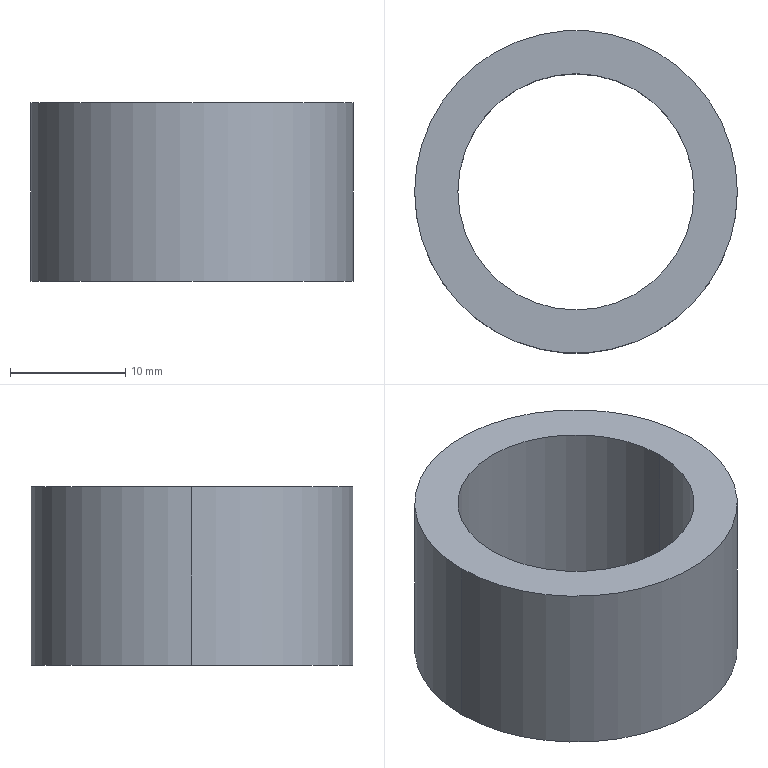Part | SolidWorks | features BaseBody 1 | 1 solid | 6 faces | box 28 x 28 x 15.5 mm | volume 4428 mm3 | cylinder 4 | plane 2 | commonest cylinder face diameters 20.5 x2 28 x2
STEP:
#1=CARTESIAN_POINT('',(10.25,0.,15.5));
#2=VERTEX_POINT('',#1);
#3=CARTESIAN_POINT('',(10.25,0.,0.));
#4=VERTEX_POINT('',#3);
#5=CARTESIAN_POINT('',(10.25,0.,15.5));
#6=DIRECTION('',(0.,0.,-1.));
#7=VECTOR('',#6,1000.);
#8=LINE('',#5,#7);
#9=EDGE_CURVE('',#2,#4,#8,.T.);
#10=ORIENTED_EDGE('',*,*,#9,.F.);
#11=CARTESIAN_POINT('',(-10.25,0.,15.5));
#12=VERTEX_POINT('',#11);
#13=CARTESIAN_POINT('',(0.,0.,15.5));
#14=DIRECTION('',(0.,0.,1.));
#15=DIRECTION('',(1.,0.,0.));
#16=AXIS2_PLACEMENT_3D('',#13,#14,#15);
#17=CIRCLE('',#16,10.25);
#18=EDGE_CURVE('',#2,#12,#17,.T.);
#19=ORIENTED_EDGE('',*,*,#18,.T.);
#20=CARTESIAN_POINT('',(-10.25,0.,0.));
#21=VERTEX_POINT('',#20);
#22=CARTESIAN_POINT('',(-10.25,0.,15.5));
#23=DIRECTION('',(0.,0.,-1.));
#24=VECTOR('',#23,1000.);
#25=LINE('',#22,#24);
#26=EDGE_CURVE('',#12,#21,#25,.T.);
#27=ORIENTED_EDGE('',*,*,#26,.T.);
#28=CARTESIAN_POINT('',(0.,0.,0.));
#29=DIRECTION('',(0.,0.,1.));
#30=DIRECTION('',(1.,0.,0.));
#31=AXIS2_PLACEMENT_3D('',#28,#29,#30);
#32=CIRCLE('',#31,10.25);
#33=EDGE_CURVE('',#4,#21,#32,.T.);
#34=ORIENTED_EDGE('',*,*,#33,.F.);
#35=EDGE_LOOP('',(#10,#19,#27,#34));
#36=FACE_OUTER_BOUND('',#35,.T.);
#37=CARTESIAN_POINT('',(0.,0.,15.5));
#38=DIRECTION('',(0.,0.,-1.));
#39=DIRECTION('',(-1.,0.,0.));
#40=AXIS2_PLACEMENT_3D('',#37,#38,#39);
#41=CYLINDRICAL_SURFACE('',#40,10.25);
#42=ADVANCED_FACE('',(#36),#41,.F.);
#43=CARTESIAN_POINT('',(14.,0.,15.5));
#44=VERTEX_POINT('',#43);
#45=CARTESIAN_POINT('',(14.,0.,0.));
#46=VERTEX_POINT('',#45);
#47=CARTESIAN_POINT('',(14.,0.,15.5));
#48=DIRECTION('',(0.,0.,-1.));
#49=VECTOR('',#48,1000.);
#50=LINE('',#47,#49);
#51=EDGE_CURVE('',#44,#46,#50,.T.);
#52=ORIENTED_EDGE('',*,*,#51,.F.);
#53=CARTESIAN_POINT('',(-14.,0.,15.5));
#54=VERTEX_POINT('',#53);
#55=CARTESIAN_POINT('',(0.,0.,15.5));
#56=DIRECTION('',(0.,0.,1.));
#57=DIRECTION('',(1.,0.,0.));
#58=AXIS2_PLACEMENT_3D('',#55,#56,#57);
#59=CIRCLE('',#58,14.);
#60=EDGE_CURVE('',#54,#44,#59,.T.);
#61=ORIENTED_EDGE('',*,*,#60,.F.);
#62=CARTESIAN_POINT('',(-14.,0.,0.));
#63=VERTEX_POINT('',#62);
#64=CARTESIAN_POINT('',(-14.,0.,15.5));
#65=DIRECTION('',(0.,0.,-1.));
#66=VECTOR('',#65,1000.);
#67=LINE('',#64,#66);
#68=EDGE_CURVE('',#54,#63,#67,.T.);
#69=ORIENTED_EDGE('',*,*,#68,.T.);
#70=CARTESIAN_POINT('',(0.,0.,0.));
#71=DIRECTION('',(0.,0.,1.));
#72=DIRECTION('',(1.,0.,0.));
#73=AXIS2_PLACEMENT_3D('',#70,#71,#72);
#74=CIRCLE('',#73,14.);
#75=EDGE_CURVE('',#63,#46,#74,.T.);
#76=ORIENTED_EDGE('',*,*,#75,.T.);
#77=EDGE_LOOP('',(#52,#61,#69,#76));
#78=FACE_OUTER_BOUND('',#77,.T.);
#79=CARTESIAN_POINT('',(0.,0.,15.5));
#80=DIRECTION('',(0.,0.,-1.));
#81=DIRECTION('',(-1.,0.,0.));
#82=AXIS2_PLACEMENT_3D('',#79,#80,#81);
#83=CYLINDRICAL_SURFACE('',#82,14.);
#84=ADVANCED_FACE('',(#78),#83,.T.);
#85=CARTESIAN_POINT('',(0.,0.,0.));
#86=DIRECTION('',(0.,0.,1.));
#87=DIRECTION('',(1.,0.,0.));
#88=AXIS2_PLACEMENT_3D('',#85,#86,#87);
#89=CIRCLE('',#88,10.25);
#90=EDGE_CURVE('',#21,#4,#89,.T.);
#91=ORIENTED_EDGE('',*,*,#90,.T.);
#92=ORIENTED_EDGE('',*,*,#33,.T.);
#93=EDGE_LOOP('',(#91,#92));
#94=FACE_BOUND('',#93,.T.);
#95=ORIENTED_EDGE('',*,*,#75,.F.);
#96=CARTESIAN_POINT('',(0.,0.,0.));
#97=DIRECTION('',(0.,0.,1.));
#98=DIRECTION('',(1.,0.,0.));
#99=AXIS2_PLACEMENT_3D('',#96,#97,#98);
#100=CIRCLE('',#99,14.);
#101=EDGE_CURVE('',#46,#63,#100,.T.);
#102=ORIENTED_EDGE('',*,*,#101,.F.);
#103=EDGE_LOOP('',(#95,#102));
#104=FACE_OUTER_BOUND('',#103,.T.);
#105=CARTESIAN_POINT('',(0.,0.,0.));
#106=DIRECTION('',(0.,0.,1.));
#107=DIRECTION('',(1.,0.,0.));
#108=AXIS2_PLACEMENT_3D('',#105,#106,#107);
#109=PLANE('',#108);
#110=ADVANCED_FACE('',(#94,#104),#109,.F.);
#111=CARTESIAN_POINT('',(0.,0.,15.5));
#112=DIRECTION('',(0.,0.,1.));
#113=DIRECTION('',(1.,0.,0.));
#114=AXIS2_PLACEMENT_3D('',#111,#112,#113);
#115=CIRCLE('',#114,10.25);
#116=EDGE_CURVE('',#12,#2,#115,.T.);
#117=ORIENTED_EDGE('',*,*,#116,.F.);
#118=ORIENTED_EDGE('',*,*,#18,.F.);
#119=EDGE_LOOP('',(#117,#118));
#120=FACE_BOUND('',#119,.T.);
#121=ORIENTED_EDGE('',*,*,#60,.T.);
#122=CARTESIAN_POINT('',(0.,0.,15.5));
#123=DIRECTION('',(0.,0.,1.));
#124=DIRECTION('',(1.,0.,0.));
#125=AXIS2_PLACEMENT_3D('',#122,#123,#124);
#126=CIRCLE('',#125,14.);
#127=EDGE_CURVE('',#44,#54,#126,.T.);
#128=ORIENTED_EDGE('',*,*,#127,.T.);
#129=EDGE_LOOP('',(#121,#128));
#130=FACE_OUTER_BOUND('',#129,.T.);
#131=CARTESIAN_POINT('',(0.,0.,15.5));
#132=DIRECTION('',(0.,0.,1.));
#133=DIRECTION('',(1.,0.,0.));
#134=AXIS2_PLACEMENT_3D('',#131,#132,#133);
#135=PLANE('',#134);
#136=ADVANCED_FACE('',(#120,#130),#135,.T.);
#137=ORIENTED_EDGE('',*,*,#127,.F.);
#138=ORIENTED_EDGE('',*,*,#51,.T.);
#139=ORIENTED_EDGE('',*,*,#101,.T.);
#140=ORIENTED_EDGE('',*,*,#68,.F.);
#141=EDGE_LOOP('',(#137,#138,#139,#140));
#142=FACE_OUTER_BOUND('',#141,.T.);
#143=CARTESIAN_POINT('',(0.,0.,15.5));
#144=DIRECTION('',(0.,0.,-1.));
#145=DIRECTION('',(-1.,0.,0.));
#146=AXIS2_PLACEMENT_3D('',#143,#144,#145);
#147=CYLINDRICAL_SURFACE('',#146,14.);
#148=ADVANCED_FACE('',(#142),#147,.T.);
#149=ORIENTED_EDGE('',*,*,#116,.T.);
#150=ORIENTED_EDGE('',*,*,#9,.T.);
#151=ORIENTED_EDGE('',*,*,#90,.F.);
#152=ORIENTED_EDGE('',*,*,#26,.F.);
#153=EDGE_LOOP('',(#149,#150,#151,#152));
#154=FACE_OUTER_BOUND('',#153,.T.);
#155=CARTESIAN_POINT('',(0.,0.,15.5));
#156=DIRECTION('',(0.,0.,-1.));
#157=DIRECTION('',(-1.,0.,0.));
#158=AXIS2_PLACEMENT_3D('',#155,#156,#157);
#159=CYLINDRICAL_SURFACE('',#158,10.25);
#160=ADVANCED_FACE('',(#154),#159,.F.);
#161=CLOSED_SHELL('',(#42,#84,#110,#136,#148,#160));
#162=MANIFOLD_SOLID_BREP('',#161);
#163=CARTESIAN_POINT('',(0.,0.,0.));
#164=DIRECTION('',(0.,0.,1.));
#165=DIRECTION('',(1.,0.,0.));
#166=AXIS2_PLACEMENT_3D('',#163,#164,#165);
#167=(LENGTH_UNIT()NAMED_UNIT(*)SI_UNIT(.MILLI.,.METRE.));
#168=UNCERTAINTY_MEASURE_WITH_UNIT(LENGTH_MEASURE(0.00001),#167,'','');
#169=(NAMED_UNIT(*)PLANE_ANGLE_UNIT()SI_UNIT($,.RADIAN.));
#170=(NAMED_UNIT(*)SI_UNIT($,.STERADIAN.)SOLID_ANGLE_UNIT());
#171=(GEOMETRIC_REPRESENTATION_CONTEXT(3)GLOBAL_UNCERTAINTY_ASSIGNED_CONTEXT((#168))GLOBAL_UNIT_ASSIGNED_CONTEXT((#167,#169,#170))REPRESENTATION_CONTEXT('',''));
#172=ADVANCED_BREP_SHAPE_REPRESENTATION('',(#162,#166),#171);